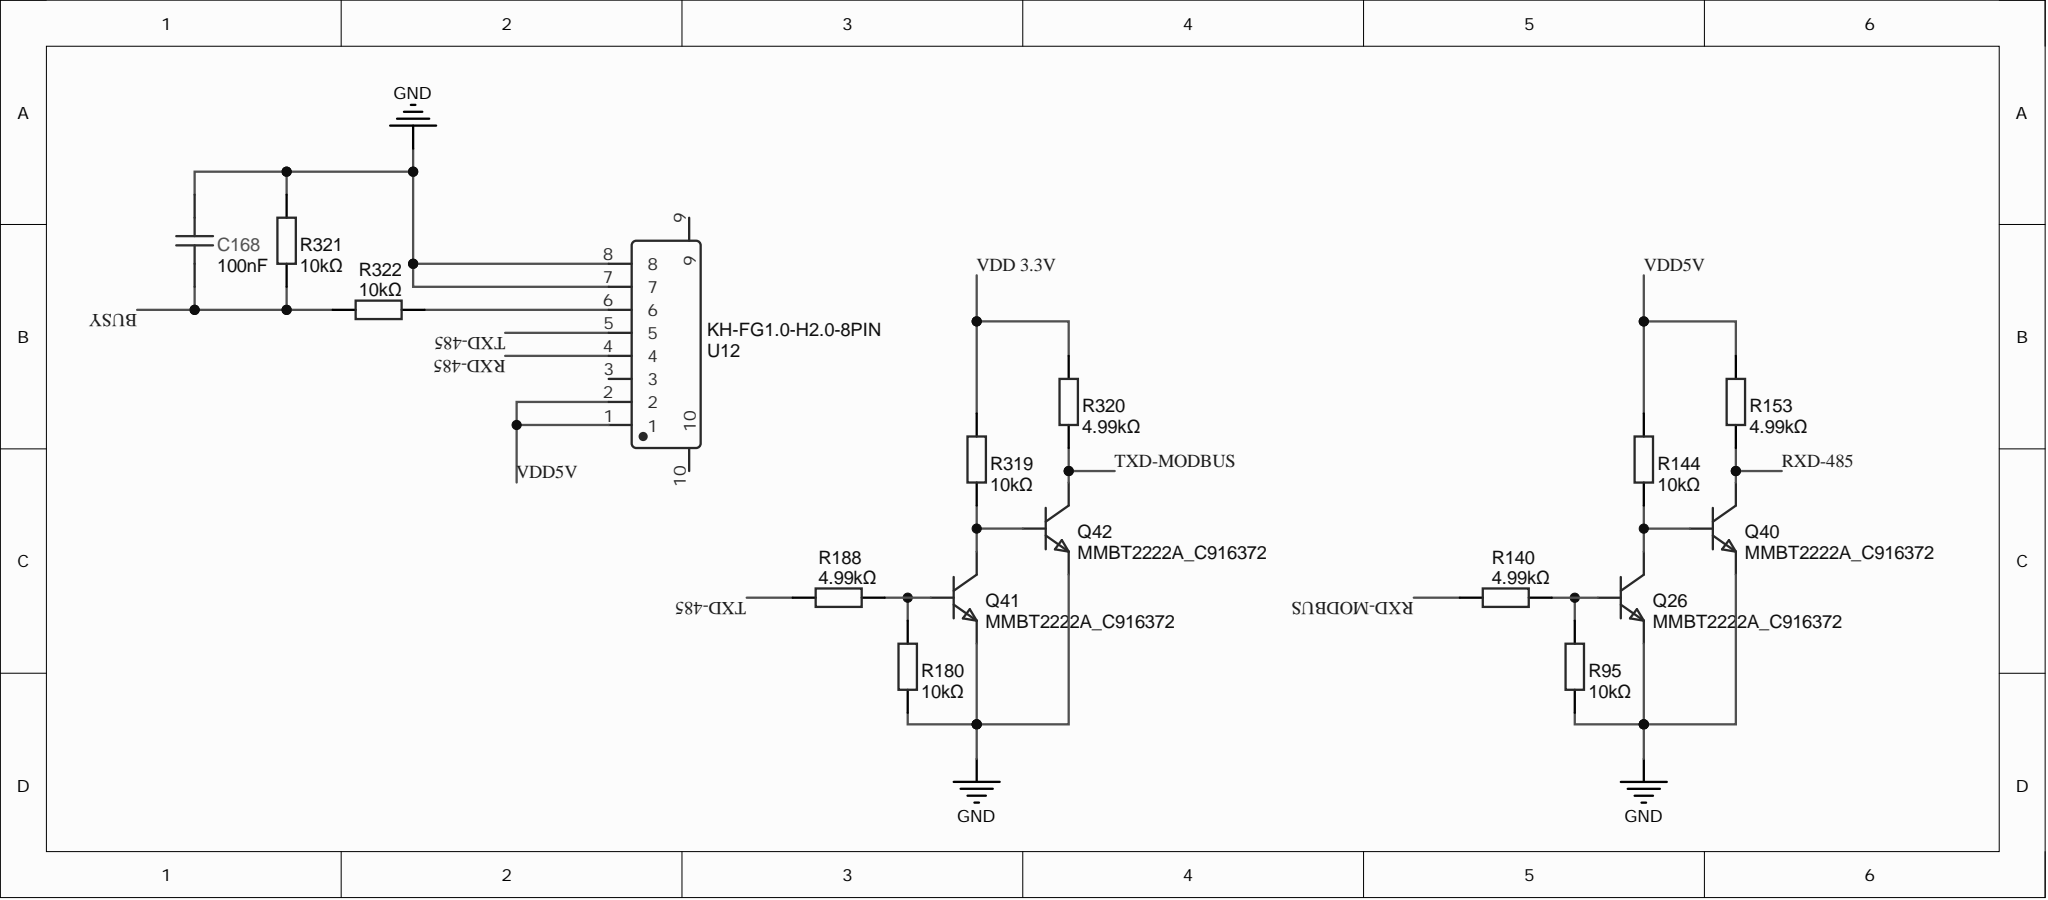Circuit board | Altium Designer | 694 parts | 423 nets | one sheet of the schematic
Parts on this sheet (reference | value | footprint):
C168 | 100nF | C0603
Q26 | MMBT2222A_C916372 | SOT-23-3_L2.9-W1.3-P1.90-LS2.4-BR
Q40 | MMBT2222A_C916372 | SOT-23-3_L2.9-W1.3-P1.90-LS2.4-BR
Q41 | MMBT2222A_C916372 | SOT-23-3_L2.9-W1.3-P1.90-LS2.4-BR
Q42 | MMBT2222A_C916372 | SOT-23-3_L2.9-W1.3-P1.90-LS2.4-BR
R95 | 10kΩ | R0603
R140 | 4.99kΩ | R0603
R144 | 10kΩ | R0603
R153 | 4.99kΩ | R0603
R180 | 10kΩ | R0603
R188 | 4.99kΩ | R0603
R319 | 10kΩ | R0603
R320 | 4.99kΩ | R0603
R321 | 10kΩ | R0603
R322 | 10kΩ | R0603
U12 | KH-FG1.0-H2.0-8PIN | FPC-SMD_KH-FG1.0-H2.0-8PIN
Nets of these parts (net: part-pin ...):
VDD 3.3V: R319-2 R320-2
VDD5V: R144-2 R153-2 U12-1 U12-2
TXD-MODBUS: Q42-3 R320-1
TXD-485: R188-2 U12-5
RXD-MODBUS: R140-1
RXD-485: Q40-3 R153-1 U12-4
NetR322_1: R322-1 U12-6
NetQ41_3: Q41-3 Q42-1 R319-1
NetQ41_1: Q41-1 R180-2 R188-1
NetQ26_3: Q26-3 Q40-1 R144-1
NetQ26_1: Q26-1 R95-2 R140-2
GND: C168-1 Q26-2 Q40-2 Q41-2 Q42-2 R95-1 R180-1 R321-2 U12-7 U12-8
BUSY: C168-2 R321-1 R322-2